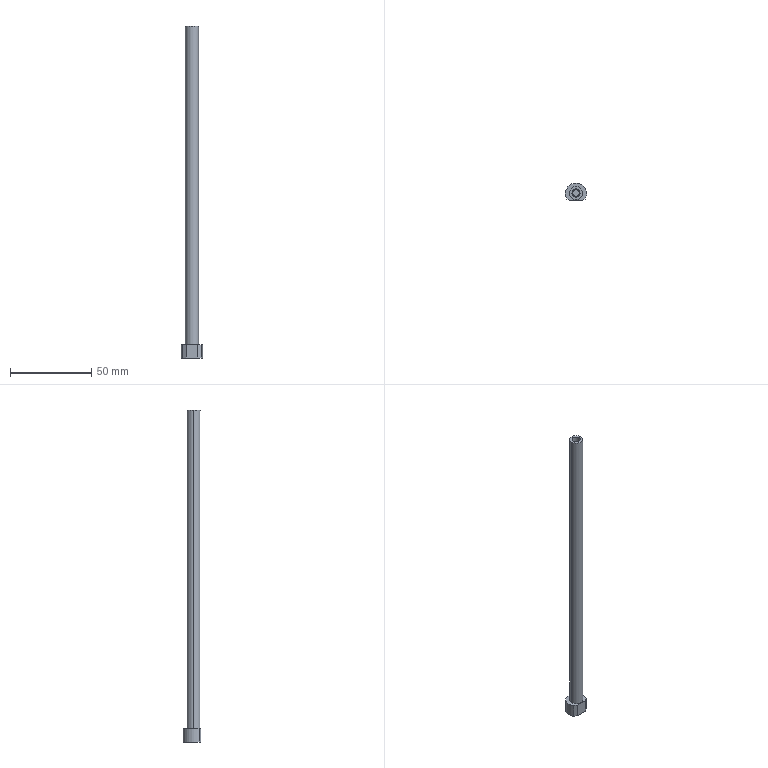Part | Creo | 1 solid | 15 faces | box 13 x 11 x 203.737 mm | volume 10572 mm3 | plane 8 | cylinder 7 | commonest cylinder face diameters 4 x2 5 x2 8 x2 13 x1
STEP:
#1=CARTESIAN_POINT('',(0.,0.,0.));
#2=DIRECTION('',(0.,0.,1.));
#3=DIRECTION('',(1.,0.,0.));
#4=AXIS2_PLACEMENT_3D('',#1,#2,#3);
#5=CARTESIAN_POINT('',(12.,94.22,-21.763));
#6=VERTEX_POINT('',#5);
#7=CARTESIAN_POINT('',(20.,94.22,-21.763));
#8=VERTEX_POINT('',#7);
#9=CARTESIAN_POINT('',(16.,94.22,-21.763));
#10=DIRECTION('',(0.,0.,1.));
#11=DIRECTION('',(-1.,0.,0.));
#12=AXIS2_PLACEMENT_3D('',#9,#10,#11);
#13=CIRCLE('',#12,4.);
#14=EDGE_CURVE('',#6,#8,#13,.T.);
#15=ORIENTED_EDGE('',*,*,#14,.F.);
#16=CARTESIAN_POINT('',(16.,94.22,-21.763));
#17=DIRECTION('',(0.,0.,1.));
#18=DIRECTION('',(1.,0.,0.));
#19=AXIS2_PLACEMENT_3D('',#16,#17,#18);
#20=CIRCLE('',#19,4.);
#21=EDGE_CURVE('',#8,#6,#20,.T.);
#22=ORIENTED_EDGE('',*,*,#21,.F.);
#23=EDGE_LOOP('',(#15,#22));
#24=FACE_OUTER_BOUND('',#23,.F.);
#25=CARTESIAN_POINT('',(13.5,94.22,-21.763));
#26=VERTEX_POINT('',#25);
#27=CARTESIAN_POINT('',(18.5,94.22,-21.763));
#28=VERTEX_POINT('',#27);
#29=CARTESIAN_POINT('',(16.,94.22,-21.763));
#30=DIRECTION('',(0.,0.,-1.));
#31=DIRECTION('',(-1.,0.,0.));
#32=AXIS2_PLACEMENT_3D('',#29,#30,#31);
#33=CIRCLE('',#32,2.5);
#34=EDGE_CURVE('',#26,#28,#33,.T.);
#35=ORIENTED_EDGE('',*,*,#34,.F.);
#36=CARTESIAN_POINT('',(16.,94.22,-21.763));
#37=DIRECTION('',(0.,0.,-1.));
#38=DIRECTION('',(1.,0.,0.));
#39=AXIS2_PLACEMENT_3D('',#36,#37,#38);
#40=CIRCLE('',#39,2.5);
#41=EDGE_CURVE('',#28,#26,#40,.T.);
#42=ORIENTED_EDGE('',*,*,#41,.F.);
#43=EDGE_LOOP('',(#35,#42));
#44=FACE_BOUND('',#43,.F.);
#45=CARTESIAN_POINT('',(63.922,-95.94,-21.763));
#46=DIRECTION('',(0.,0.,-1.));
#47=DIRECTION('',(0.,1.,0.));
#48=AXIS2_PLACEMENT_3D('',#45,#46,#47);
#49=PLANE('',#48);
#50=ADVANCED_FACE('',(#24,#44),#49,.F.);
#51=ORIENTED_EDGE('',*,*,#14,.T.);
#52=CARTESIAN_POINT('',(20.,94.22,-217.5));
#53=VERTEX_POINT('',#52);
#54=CARTESIAN_POINT('',(20.,94.22,-21.763));
#55=DIRECTION('',(0.,0.,-1.));
#56=VECTOR('',#55,195.737);
#57=LINE('',#54,#56);
#58=EDGE_CURVE('',#8,#53,#57,.T.);
#59=ORIENTED_EDGE('',*,*,#58,.T.);
#60=CARTESIAN_POINT('',(12.,94.22,-217.5));
#61=VERTEX_POINT('',#60);
#62=CARTESIAN_POINT('',(16.,94.22,-217.5));
#63=DIRECTION('',(0.,0.,-1.));
#64=DIRECTION('',(1.,0.,0.));
#65=AXIS2_PLACEMENT_3D('',#62,#63,#64);
#66=CIRCLE('',#65,4.);
#67=EDGE_CURVE('',#53,#61,#66,.T.);
#68=ORIENTED_EDGE('',*,*,#67,.T.);
#69=CARTESIAN_POINT('',(12.,94.22,-21.763));
#70=DIRECTION('',(0.,0.,-1.));
#71=VECTOR('',#70,195.737);
#72=LINE('',#69,#71);
#73=EDGE_CURVE('',#6,#61,#72,.T.);
#74=ORIENTED_EDGE('',*,*,#73,.F.);
#75=EDGE_LOOP('',(#51,#59,#68,#74));
#76=FACE_OUTER_BOUND('',#75,.F.);
#77=CARTESIAN_POINT('',(16.,94.22,-20.767));
#78=DIRECTION('',(0.,0.,-1.));
#79=DIRECTION('',(-1.,0.,0.));
#80=AXIS2_PLACEMENT_3D('',#77,#78,#79);
#81=CYLINDRICAL_SURFACE('',#80,4.);
#82=ADVANCED_FACE('',(#76),#81,.T.);
#83=ORIENTED_EDGE('',*,*,#21,.T.);
#84=ORIENTED_EDGE('',*,*,#73,.T.);
#85=CARTESIAN_POINT('',(16.,94.22,-217.5));
#86=DIRECTION('',(0.,0.,-1.));
#87=DIRECTION('',(-1.,0.,0.));
#88=AXIS2_PLACEMENT_3D('',#85,#86,#87);
#89=CIRCLE('',#88,4.);
#90=EDGE_CURVE('',#61,#53,#89,.T.);
#91=ORIENTED_EDGE('',*,*,#90,.T.);
#92=ORIENTED_EDGE('',*,*,#58,.F.);
#93=EDGE_LOOP('',(#83,#84,#91,#92));
#94=FACE_OUTER_BOUND('',#93,.F.);
#95=CARTESIAN_POINT('',(16.,94.22,-20.767));
#96=DIRECTION('',(0.,0.,-1.));
#97=DIRECTION('',(-1.,0.,0.));
#98=AXIS2_PLACEMENT_3D('',#95,#96,#97);
#99=CYLINDRICAL_SURFACE('',#98,4.);
#100=ADVANCED_FACE('',(#94),#99,.T.);
#101=CARTESIAN_POINT('',(12.448,89.72,-217.5));
#102=VERTEX_POINT('',#101);
#103=CARTESIAN_POINT('',(19.552,89.72,-217.5));
#104=VERTEX_POINT('',#103);
#105=CARTESIAN_POINT('',(12.448,89.72,-217.5));
#106=DIRECTION('',(1.,0.,0.));
#107=VECTOR('',#106,7.105);
#108=LINE('',#105,#107);
#109=EDGE_CURVE('',#102,#104,#108,.T.);
#110=ORIENTED_EDGE('',*,*,#109,.F.);
#111=CARTESIAN_POINT('',(10.443,90.849,-217.5));
#112=VERTEX_POINT('',#111);
#113=CARTESIAN_POINT('',(10.443,90.849,-217.5));
#114=DIRECTION('',(0.8714,-0.4906,0.));
#115=VECTOR('',#114,2.301);
#116=LINE('',#113,#115);
#117=EDGE_CURVE('',#112,#102,#116,.T.);
#118=ORIENTED_EDGE('',*,*,#117,.F.);
#119=CARTESIAN_POINT('',(22.5,94.22,-217.5));
#120=VERTEX_POINT('',#119);
#121=CARTESIAN_POINT('',(16.,94.22,-217.5));
#122=DIRECTION('',(0.,0.,1.));
#123=DIRECTION('',(1.,0.,0.));
#124=AXIS2_PLACEMENT_3D('',#121,#122,#123);
#125=CIRCLE('',#124,6.5);
#126=EDGE_CURVE('',#120,#112,#125,.T.);
#127=ORIENTED_EDGE('',*,*,#126,.F.);
#128=CARTESIAN_POINT('',(21.557,90.849,-217.5));
#129=VERTEX_POINT('',#128);
#130=CARTESIAN_POINT('',(16.,94.22,-217.5));
#131=DIRECTION('',(0.,0.,1.));
#132=DIRECTION('',(0.855,-0.5186,0.));
#133=AXIS2_PLACEMENT_3D('',#130,#131,#132);
#134=CIRCLE('',#133,6.5);
#135=EDGE_CURVE('',#129,#120,#134,.T.);
#136=ORIENTED_EDGE('',*,*,#135,.F.);
#137=CARTESIAN_POINT('',(19.552,89.72,-217.5));
#138=DIRECTION('',(0.8714,0.4906,0.));
#139=VECTOR('',#138,2.301);
#140=LINE('',#137,#139);
#141=EDGE_CURVE('',#104,#129,#140,.T.);
#142=ORIENTED_EDGE('',*,*,#141,.F.);
#143=EDGE_LOOP('',(#110,#118,#127,#136,#142));
#144=FACE_OUTER_BOUND('',#143,.F.);
#145=ORIENTED_EDGE('',*,*,#90,.F.);
#146=ORIENTED_EDGE('',*,*,#67,.F.);
#147=EDGE_LOOP('',(#145,#146));
#148=FACE_BOUND('',#147,.F.);
#149=CARTESIAN_POINT('',(32.,-1.78,-217.5));
#150=DIRECTION('',(0.,0.,-1.));
#151=DIRECTION('',(-1.,0.,0.));
#152=AXIS2_PLACEMENT_3D('',#149,#150,#151);
#153=PLANE('',#152);
#154=ADVANCED_FACE('',(#144,#148),#153,.F.);
#155=CARTESIAN_POINT('',(12.448,89.72,-225.5));
#156=VERTEX_POINT('',#155);
#157=CARTESIAN_POINT('',(19.552,89.72,-225.5));
#158=VERTEX_POINT('',#157);
#159=CARTESIAN_POINT('',(12.448,89.72,-225.5));
#160=DIRECTION('',(1.,0.,0.));
#161=VECTOR('',#160,7.105);
#162=LINE('',#159,#161);
#163=EDGE_CURVE('',#156,#158,#162,.T.);
#164=ORIENTED_EDGE('',*,*,#163,.F.);
#165=CARTESIAN_POINT('',(12.448,89.72,-225.5));
#166=DIRECTION('',(0.,0.,1.));
#167=VECTOR('',#166,8.);
#168=LINE('',#165,#167);
#169=EDGE_CURVE('',#156,#102,#168,.T.);
#170=ORIENTED_EDGE('',*,*,#169,.T.);
#171=ORIENTED_EDGE('',*,*,#109,.T.);
#172=CARTESIAN_POINT('',(19.552,89.72,-217.5));
#173=DIRECTION('',(0.,0.,-1.));
#174=VECTOR('',#173,8.);
#175=LINE('',#172,#174);
#176=EDGE_CURVE('',#104,#158,#175,.T.);
#177=ORIENTED_EDGE('',*,*,#176,.T.);
#178=EDGE_LOOP('',(#164,#170,#171,#177));
#179=FACE_OUTER_BOUND('',#178,.F.);
#180=CARTESIAN_POINT('',(16.,89.72,-221.5));
#181=DIRECTION('',(0.,-1.,0.));
#182=DIRECTION('',(0.,0.,-1.));
#183=AXIS2_PLACEMENT_3D('',#180,#181,#182);
#184=PLANE('',#183);
#185=ADVANCED_FACE('',(#179),#184,.T.);
#186=CARTESIAN_POINT('',(10.443,90.849,-225.5));
#187=VERTEX_POINT('',#186);
#188=CARTESIAN_POINT('',(22.5,94.22,-225.5));
#189=VERTEX_POINT('',#188);
#190=CARTESIAN_POINT('',(16.,94.22,-225.5));
#191=DIRECTION('',(0.,0.,-1.));
#192=DIRECTION('',(-0.855,-0.5186,0.));
#193=AXIS2_PLACEMENT_3D('',#190,#191,#192);
#194=CIRCLE('',#193,6.5);
#195=EDGE_CURVE('',#187,#189,#194,.T.);
#196=ORIENTED_EDGE('',*,*,#195,.F.);
#197=CARTESIAN_POINT('',(12.448,89.72,-225.5));
#198=DIRECTION('',(-0.8714,0.4906,0.));
#199=VECTOR('',#198,2.301);
#200=LINE('',#197,#199);
#201=EDGE_CURVE('',#156,#187,#200,.T.);
#202=ORIENTED_EDGE('',*,*,#201,.F.);
#203=ORIENTED_EDGE('',*,*,#163,.T.);
#204=CARTESIAN_POINT('',(21.557,90.849,-225.5));
#205=VERTEX_POINT('',#204);
#206=CARTESIAN_POINT('',(21.557,90.849,-225.5));
#207=DIRECTION('',(-0.8714,-0.4906,0.));
#208=VECTOR('',#207,2.301);
#209=LINE('',#206,#208);
#210=EDGE_CURVE('',#205,#158,#209,.T.);
#211=ORIENTED_EDGE('',*,*,#210,.F.);
#212=CARTESIAN_POINT('',(16.,94.22,-225.5));
#213=DIRECTION('',(0.,0.,-1.));
#214=DIRECTION('',(1.,0.,0.));
#215=AXIS2_PLACEMENT_3D('',#212,#213,#214);
#216=CIRCLE('',#215,6.5);
#217=EDGE_CURVE('',#189,#205,#216,.T.);
#218=ORIENTED_EDGE('',*,*,#217,.F.);
#219=EDGE_LOOP('',(#196,#202,#203,#211,#218));
#220=FACE_OUTER_BOUND('',#219,.F.);
#221=CARTESIAN_POINT('',(32.,-1.78,-225.5));
#222=DIRECTION('',(0.,0.,-1.));
#223=DIRECTION('',(-1.,0.,0.));
#224=AXIS2_PLACEMENT_3D('',#221,#222,#223);
#225=PLANE('',#224);
#226=ADVANCED_FACE('',(#220),#225,.T.);
#227=ORIENTED_EDGE('',*,*,#126,.T.);
#228=CARTESIAN_POINT('',(10.443,90.849,-225.5));
#229=DIRECTION('',(0.,0.,1.));
#230=VECTOR('',#229,8.);
#231=LINE('',#228,#230);
#232=EDGE_CURVE('',#187,#112,#231,.T.);
#233=ORIENTED_EDGE('',*,*,#232,.F.);
#234=ORIENTED_EDGE('',*,*,#195,.T.);
#235=ORIENTED_EDGE('',*,*,#217,.T.);
#236=CARTESIAN_POINT('',(21.557,90.849,-217.5));
#237=DIRECTION('',(0.,0.,-1.));
#238=VECTOR('',#237,8.);
#239=LINE('',#236,#238);
#240=EDGE_CURVE('',#129,#205,#239,.T.);
#241=ORIENTED_EDGE('',*,*,#240,.F.);
#242=ORIENTED_EDGE('',*,*,#135,.T.);
#243=EDGE_LOOP('',(#227,#233,#234,#235,#241,#242));
#244=FACE_OUTER_BOUND('',#243,.F.);
#245=CARTESIAN_POINT('',(16.,94.22,-225.5));
#246=DIRECTION('',(0.,0.,1.));
#247=DIRECTION('',(1.,0.,0.));
#248=AXIS2_PLACEMENT_3D('',#245,#246,#247);
#249=CYLINDRICAL_SURFACE('',#248,6.5);
#250=ADVANCED_FACE('',(#244),#249,.T.);
#251=ORIENTED_EDGE('',*,*,#201,.T.);
#252=ORIENTED_EDGE('',*,*,#232,.T.);
#253=ORIENTED_EDGE('',*,*,#117,.T.);
#254=ORIENTED_EDGE('',*,*,#169,.F.);
#255=EDGE_LOOP('',(#251,#252,#253,#254));
#256=FACE_OUTER_BOUND('',#255,.F.);
#257=CARTESIAN_POINT('',(10.443,90.849,-225.5));
#258=DIRECTION('',(0.4906,0.8714,0.));
#259=DIRECTION('',(0.,0.,1.));
#260=AXIS2_PLACEMENT_3D('',#257,#258,#259);
#261=PLANE('',#260);
#262=ADVANCED_FACE('',(#256),#261,.F.);
#263=ORIENTED_EDGE('',*,*,#141,.T.);
#264=ORIENTED_EDGE('',*,*,#240,.T.);
#265=ORIENTED_EDGE('',*,*,#210,.T.);
#266=ORIENTED_EDGE('',*,*,#176,.F.);
#267=EDGE_LOOP('',(#263,#264,#265,#266));
#268=FACE_OUTER_BOUND('',#267,.F.);
#269=CARTESIAN_POINT('',(21.557,90.849,-225.5));
#270=DIRECTION('',(0.4906,-0.8714,0.));
#271=DIRECTION('',(0.,0.,1.));
#272=AXIS2_PLACEMENT_3D('',#269,#270,#271);
#273=PLANE('',#272);
#274=ADVANCED_FACE('',(#268),#273,.T.);
#275=CARTESIAN_POINT('',(18.5,94.22,-30.763));
#276=VERTEX_POINT('',#275);
#277=CARTESIAN_POINT('',(13.5,94.22,-30.763));
#278=VERTEX_POINT('',#277);
#279=CARTESIAN_POINT('',(16.,94.22,-30.763));
#280=DIRECTION('',(0.,0.,1.));
#281=DIRECTION('',(1.,0.,0.));
#282=AXIS2_PLACEMENT_3D('',#279,#280,#281);
#283=CIRCLE('',#282,2.5);
#284=EDGE_CURVE('',#276,#278,#283,.T.);
#285=ORIENTED_EDGE('',*,*,#284,.T.);
#286=CARTESIAN_POINT('',(13.5,94.22,-21.763));
#287=DIRECTION('',(0.,0.,-1.));
#288=VECTOR('',#287,9.);
#289=LINE('',#286,#288);
#290=EDGE_CURVE('',#26,#278,#289,.T.);
#291=ORIENTED_EDGE('',*,*,#290,.F.);
#292=ORIENTED_EDGE('',*,*,#34,.T.);
#293=CARTESIAN_POINT('',(18.5,94.22,-21.763));
#294=DIRECTION('',(0.,0.,-1.));
#295=VECTOR('',#294,9.);
#296=LINE('',#293,#295);
#297=EDGE_CURVE('',#28,#276,#296,.T.);
#298=ORIENTED_EDGE('',*,*,#297,.T.);
#299=EDGE_LOOP('',(#285,#291,#292,#298));
#300=FACE_OUTER_BOUND('',#299,.F.);
#301=CARTESIAN_POINT('',(16.,94.22,-21.763));
#302=DIRECTION('',(0.,0.,-1.));
#303=DIRECTION('',(-1.,0.,0.));
#304=AXIS2_PLACEMENT_3D('',#301,#302,#303);
#305=CYLINDRICAL_SURFACE('',#304,2.5);
#306=ADVANCED_FACE('',(#300),#305,.F.);
#307=CARTESIAN_POINT('',(16.,94.22,-30.763));
#308=DIRECTION('',(0.,0.,1.));
#309=DIRECTION('',(-1.,0.,0.));
#310=AXIS2_PLACEMENT_3D('',#307,#308,#309);
#311=CIRCLE('',#310,2.5);
#312=EDGE_CURVE('',#278,#276,#311,.T.);
#313=ORIENTED_EDGE('',*,*,#312,.F.);
#314=ORIENTED_EDGE('',*,*,#284,.F.);
#315=EDGE_LOOP('',(#313,#314));
#316=FACE_OUTER_BOUND('',#315,.F.);
#317=CARTESIAN_POINT('',(14.,94.22,-30.763));
#318=VERTEX_POINT('',#317);
#319=CARTESIAN_POINT('',(18.,94.22,-30.763));
#320=VERTEX_POINT('',#319);
#321=CARTESIAN_POINT('',(16.,94.22,-30.763));
#322=DIRECTION('',(0.,0.,-1.));
#323=DIRECTION('',(-1.,0.,0.));
#324=AXIS2_PLACEMENT_3D('',#321,#322,#323);
#325=CIRCLE('',#324,2.);
#326=EDGE_CURVE('',#318,#320,#325,.T.);
#327=ORIENTED_EDGE('',*,*,#326,.F.);
#328=CARTESIAN_POINT('',(16.,94.22,-30.763));
#329=DIRECTION('',(0.,0.,-1.));
#330=DIRECTION('',(1.,0.,0.));
#331=AXIS2_PLACEMENT_3D('',#328,#329,#330);
#332=CIRCLE('',#331,2.);
#333=EDGE_CURVE('',#320,#318,#332,.T.);
#334=ORIENTED_EDGE('',*,*,#333,.F.);
#335=EDGE_LOOP('',(#327,#334));
#336=FACE_BOUND('',#335,.F.);
#337=CARTESIAN_POINT('',(16.,94.22,-30.763));
#338=DIRECTION('',(0.,0.,-1.));
#339=DIRECTION('',(-1.,0.,0.));
#340=AXIS2_PLACEMENT_3D('',#337,#338,#339);
#341=PLANE('',#340);
#342=ADVANCED_FACE('',(#316,#336),#341,.F.);
#343=ORIENTED_EDGE('',*,*,#326,.T.);
#344=CARTESIAN_POINT('',(18.,94.22,-33.763));
#345=VERTEX_POINT('',#344);
#346=CARTESIAN_POINT('',(18.,94.22,-30.763));
#347=DIRECTION('',(0.,0.,-1.));
#348=VECTOR('',#347,3.);
#349=LINE('',#346,#348);
#350=EDGE_CURVE('',#320,#345,#349,.T.);
#351=ORIENTED_EDGE('',*,*,#350,.T.);
#352=CARTESIAN_POINT('',(14.,94.22,-33.763));
#353=VERTEX_POINT('',#352);
#354=CARTESIAN_POINT('',(16.,94.22,-33.763));
#355=DIRECTION('',(0.,0.,1.));
#356=DIRECTION('',(1.,0.,0.));
#357=AXIS2_PLACEMENT_3D('',#354,#355,#356);
#358=CIRCLE('',#357,2.);
#359=EDGE_CURVE('',#345,#353,#358,.T.);
#360=ORIENTED_EDGE('',*,*,#359,.T.);
#361=CARTESIAN_POINT('',(14.,94.22,-30.763));
#362=DIRECTION('',(0.,0.,-1.));
#363=VECTOR('',#362,3.);
#364=LINE('',#361,#363);
#365=EDGE_CURVE('',#318,#353,#364,.T.);
#366=ORIENTED_EDGE('',*,*,#365,.F.);
#367=EDGE_LOOP('',(#343,#351,#360,#366));
#368=FACE_OUTER_BOUND('',#367,.F.);
#369=CARTESIAN_POINT('',(16.,94.22,-21.763));
#370=DIRECTION('',(0.,0.,-1.));
#371=DIRECTION('',(-1.,0.,0.));
#372=AXIS2_PLACEMENT_3D('',#369,#370,#371);
#373=CYLINDRICAL_SURFACE('',#372,2.);
#374=ADVANCED_FACE('',(#368),#373,.F.);
#375=ORIENTED_EDGE('',*,*,#333,.T.);
#376=ORIENTED_EDGE('',*,*,#365,.T.);
#377=CARTESIAN_POINT('',(16.,94.22,-33.763));
#378=DIRECTION('',(0.,0.,1.));
#379=DIRECTION('',(-1.,0.,0.));
#380=AXIS2_PLACEMENT_3D('',#377,#378,#379);
#381=CIRCLE('',#380,2.);
#382=EDGE_CURVE('',#353,#345,#381,.T.);
#383=ORIENTED_EDGE('',*,*,#382,.T.);
#384=ORIENTED_EDGE('',*,*,#350,.F.);
#385=EDGE_LOOP('',(#375,#376,#383,#384));
#386=FACE_OUTER_BOUND('',#385,.F.);
#387=CARTESIAN_POINT('',(16.,94.22,-21.763));
#388=DIRECTION('',(0.,0.,-1.));
#389=DIRECTION('',(-1.,0.,0.));
#390=AXIS2_PLACEMENT_3D('',#387,#388,#389);
#391=CYLINDRICAL_SURFACE('',#390,2.);
#392=ADVANCED_FACE('',(#386),#391,.F.);
#393=ORIENTED_EDGE('',*,*,#382,.F.);
#394=ORIENTED_EDGE('',*,*,#359,.F.);
#395=EDGE_LOOP('',(#393,#394));
#396=FACE_OUTER_BOUND('',#395,.F.);
#397=CARTESIAN_POINT('',(16.,94.22,-33.763));
#398=DIRECTION('',(0.,0.,-1.));
#399=DIRECTION('',(-1.,0.,0.));
#400=AXIS2_PLACEMENT_3D('',#397,#398,#399);
#401=PLANE('',#400);
#402=ADVANCED_FACE('',(#396),#401,.F.);
#403=ORIENTED_EDGE('',*,*,#312,.T.);
#404=ORIENTED_EDGE('',*,*,#297,.F.);
#405=ORIENTED_EDGE('',*,*,#41,.T.);
#406=ORIENTED_EDGE('',*,*,#290,.T.);
#407=EDGE_LOOP('',(#403,#404,#405,#406));
#408=FACE_OUTER_BOUND('',#407,.F.);
#409=CARTESIAN_POINT('',(16.,94.22,-21.763));
#410=DIRECTION('',(0.,0.,-1.));
#411=DIRECTION('',(-1.,0.,0.));
#412=AXIS2_PLACEMENT_3D('',#409,#410,#411);
#413=CYLINDRICAL_SURFACE('',#412,2.5);
#414=ADVANCED_FACE('',(#408),#413,.F.);
#415=CLOSED_SHELL('',(#50,#82,#100,#154,#185,#226,#250,#262,#274,#306,#342,#374,#392,#402,#414));
#416=MANIFOLD_SOLID_BREP('',#415);
#417=(LENGTH_UNIT()NAMED_UNIT(*)SI_UNIT(.MILLI.,.METRE.));
#418=UNCERTAINTY_MEASURE_WITH_UNIT(LENGTH_MEASURE(0.02044),#417,'','');
#419=(NAMED_UNIT(*)PLANE_ANGLE_UNIT()SI_UNIT($,.RADIAN.));
#420=PLANE_ANGLE_MEASURE_WITH_UNIT(PLANE_ANGLE_MEASURE(0.01745),#419);
#421=(CONVERSION_BASED_UNIT('DEGREE',#420)NAMED_UNIT(*)PLANE_ANGLE_UNIT());
#422=(NAMED_UNIT(*)SI_UNIT($,.STERADIAN.)SOLID_ANGLE_UNIT());
#423=(GEOMETRIC_REPRESENTATION_CONTEXT(3)GLOBAL_UNCERTAINTY_ASSIGNED_CONTEXT((#418))GLOBAL_UNIT_ASSIGNED_CONTEXT((#417,#421,#422))REPRESENTATION_CONTEXT('',''));
#424=ADVANCED_BREP_SHAPE_REPRESENTATION('',(#4,#416),#423);